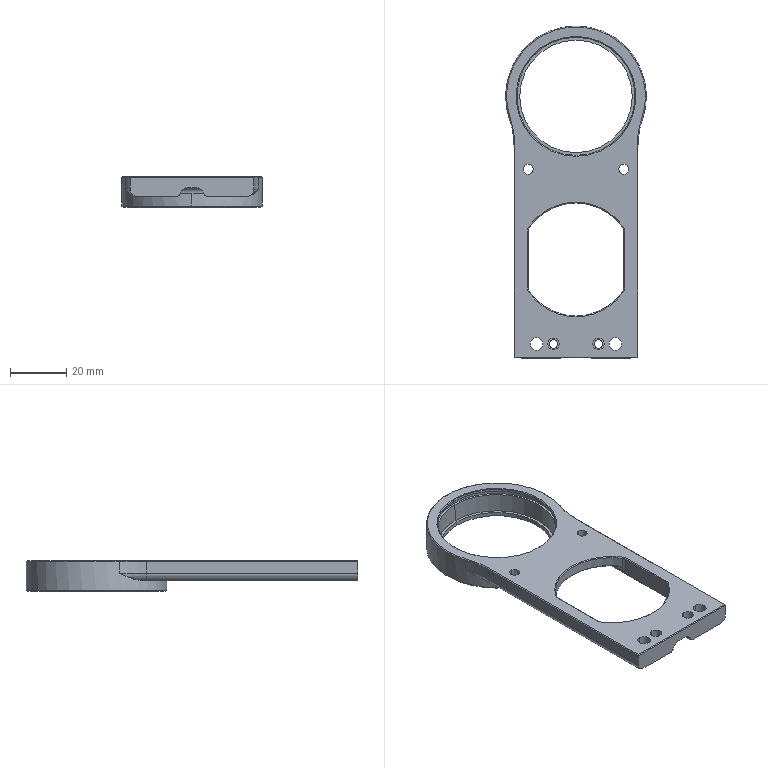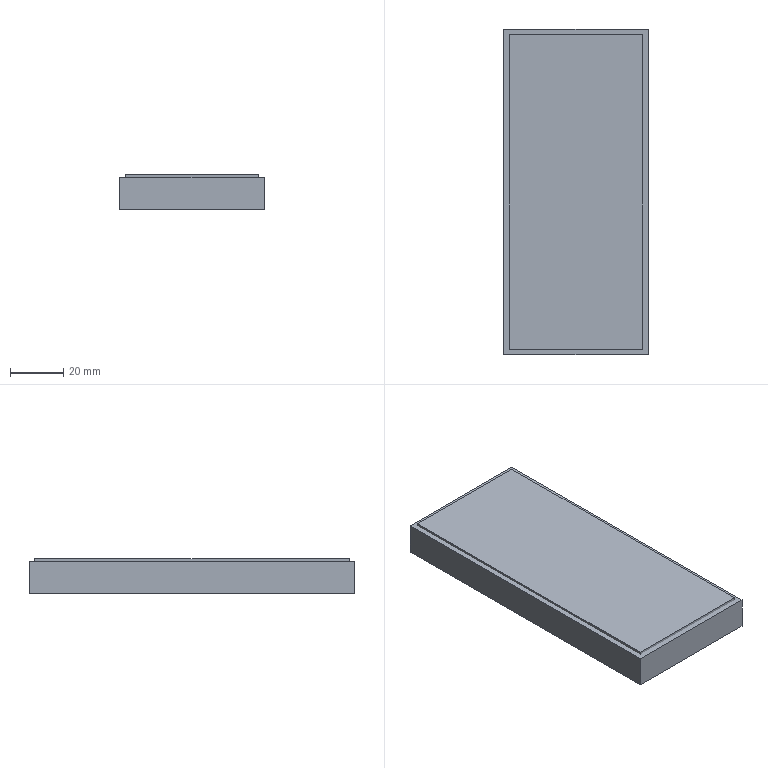CAM job | NX | 3-axis milling, drilling | part box 50 x 118 x 11 mm | stock box 54 x 122 x 13 mm
Tools:
number,name,description,diameter,corner_radius,flute_length,length,flutes
19,D80,Milling Tool-5 Parameters,80.0,0.0,50.0,75.0,2
15,D10,Milling Tool-5 Parameters,10.0,0.0,50.0,75.0,2
14,D10JING,Milling Tool-5 Parameters,10.0,0.0,50.0,75.0,2
1,D6A45,Milling Tool-5 Parameters,6.0,0.0,50.0,75.0,2
8,4.5ZT,Drilling Tool,4.5,0.0,35.0,50.0,2
16,3.0ZT,Drilling Tool,3.0,0.0,35.0,50.0,2
7,3.5ZT,Drilling Tool,3.4,0.0,35.0,50.0,2
17,D2,Milling Tool-5 Parameters,2.0,0.0,50.0,75.0,2
11,D4,Milling Tool-5 Parameters,4.0,0.0,50.0,75.0,2
18,D3R0.5,Milling Tool-5 Parameters,3.0,0.5,50.0,75.0,2
21,T6H4D1.5,Milling Tool-T Cutter,6.0,,1.5,25.0,4
Operations:
program,operation,operation_type,tool,method,geometry_group,spindle_rpm,surface_speed,feed_per_tooth,feed_cut,feed_plunge,cut_length_mm,path_length_mm,cut_time_min,machine_time_min
1,FLOOR_WALL,VolumeBased25DMillingOperation,D80,METHOD,A,5000.0,1256.0,0.12,1200.0,100.0,214.0,268.0,0.1783,0.1837
1,ZLEVEL_PROFILE,ZLevelMilling,D10,METHOD,A,9500.0,298.0,0.1842,3500.0,1000.0,4822.763,4890.763,1.409,1.416
1,PLANAR_MILL_3,PlanarMilling,D10,METHOD,A,9500.0,298.0,0.1842,3500.0,1000.0,2427.202,2623.254,1.069,1.088
1,HOLE_MILLING_COPY,CylinderMilling,D10,METHOD,A,9500.0,0.0,0.0,2500.0,1000.0,990.111,1061.111,0.3984,0.4055
1,ZLEVEL_PROFILE_COPY,ZLevelMilling,D10JING,METHOD,A,9500.0,298.0,0.0789,1500.0,1000.0,370.783,449.783,0.2567,0.2646
1,ZLEVEL_PROFILE_COPY_1_COPY,ZLevelMilling,D10JING,METHOD,A,9500.0,298.0,0.0789,1500.0,1000.0,122.302,200.302,0.0911,0.0989
1,HOLE_MILLING_COPY_COPY,CylinderMilling,D10JING,METHOD,A,9500.0,0.0,0.1053,2000.0,1000.0,1159.087,1228.112,0.5921,0.599
1,HOLE_MILLING_COPY_COPY_COPY,CylinderMilling,D10JING,METHOD,A,9500.0,0.0,0.1053,2000.0,1000.0,264.056,324.806,0.1413,0.1474
1,SPOT_DRILLING,Operation,D6A45,METHOD,A,9500.0,179.0,0.0132,250.0,0.0,28.0,288.202,0.112,0.138
1,DRILLING,Operation,4.5ZT,METHOD,A,2500.0,35.0,0.04,200.0,0.0,18.904,128.968,0.0945,0.1055
1,DRILLING_COPY,Operation,3.0ZT,METHOD,A,2500.0,35.0,0.04,200.0,0.0,24.803,128.884,0.124,0.1344
1,DRILLING_COPY_COPY,Operation,3.5ZT,METHOD,A,2500.0,35.0,0.04,200.0,0.0,25.043,147.218,0.1252,0.1374
1,ZLEVEL_PROFILE_COPY_1_COPY_1,ZLevelMilling,D4,METHOD,A,9500.0,119.0,0.1053,2000.0,1000.0,727.717,1313.287,0.5001,0.5587
1,HOLE_MILLING_1,CylinderMilling,D2,METHOD,A,9500.0,59.0,0.0553,1050.0,100.0,479.748,624.748,0.4569,0.4714
1,PLANAR_PROFILE,PlanarMilling,D6A45,METHOD,A,9500.0,179.0,0.0789,1500.0,100.0,577.995,865.461,0.3853,0.4141
1,PLANAR_PROFILE_COPY,PlanarMilling,D6A45,METHOD,A,9500.0,179.0,0.0789,1500.0,100.0,81.045,559.42,0.054,0.1019
1,PLANAR_MILL,PlanarMilling,T6H4D1.5,METHOD,A,9500.0,179.0,0.0329,1250.0,100.0,366.114,425.114,0.2929,0.2988
2,FLOOR_WALL_COPY,VolumeBased25DMillingOperation,D80,METHOD,B,5000.0,1256.0,0.12,1200.0,100.0,428.0,741.7,0.3567,0.388
2,FLOOR_WALL_COPY_COPY,VolumeBased25DMillingOperation,D80,METHOD,B,5000.0,1256.0,0.12,1200.0,100.0,214.0,268.0,0.1783,0.1837
2,FLOOR_WALL_1,VolumeBased25DMillingOperation,D10,METHOD,B,9500.0,298.0,0.1316,2500.0,1000.0,4682.065,4846.9,2.015,2.031
2,FLOOR_WALL_1_COPY,VolumeBased25DMillingOperation,D10,METHOD,B,9500.0,298.0,0.1316,2500.0,1000.0,934.411,1180.147,0.5939,0.6185
2,FLOOR_WALL_1_COPY_1_COPY_COPY,VolumeBased25DMillingOperation,D10JING,METHOD,B,9500.0,119.0,0.0632,1200.0,1000.0,1053.375,1671.004,0.8821,0.9438
2,HOLE_MILLING_2,CylinderMilling,D4,METHOD,B,9500.0,119.0,0.0658,1250.0,100.0,212.223,382.023,0.1698,0.1868
2,FLOOR_WALL_1_COPY_1,VolumeBased25DMillingOperation,D4,METHOD,B,9500.0,119.0,0.1053,2000.0,1000.0,865.886,1629.214,0.5963,0.6726
2,ZLEVEL_PROFILE_1_COPY,ZLevelMilling,D3R0.5,METHOD,B,9500.0,89.0,0.1316,2500.0,1000.0,26172.752,26608.685,10.485,10.528
2,ZLEVEL_PROFILE_1_COPY_COPY,ZLevelMilling,D3R0.5,METHOD,B,9500.0,89.0,0.1316,2500.0,1000.0,1212.83,1790.067,0.5077,0.5654
2,ZLEVEL_PROFILE_1_COPY_COPY_COPY,ZLevelMilling,D3R0.5,METHOD,B,9500.0,89.0,0.1316,2500.0,1000.0,7760.246,8077.341,3.117,3.148
2,PLANAR_MILL_2,PlanarMilling,D6A45,METHOD,B,9500.0,179.0,0.0658,1250.0,100.0,126.515,185.515,0.1012,0.1071
2,PLANAR_MILL_2_COPY,PlanarMilling,D6A45,METHOD,B,9500.0,179.0,0.0658,1250.0,100.0,166.864,225.864,0.1335,0.1394
2,PLANAR_MILL_2_COPY_1,PlanarMilling,D6A45,METHOD,B,9500.0,179.0,0.0658,1250.0,100.0,122.186,802.801,0.0977,0.1658
PROGRAM,PLANAR_MILL_1,PlanarMilling,D6A45,METHOD,NONE,9500.0,179.0,0.0658,1250.0,100.0,0.0,0.0,0.0,0.0,missing
PROGRAM,ZLEVEL_PROFILE_COPY_1,ZLevelMilling,D10,METHOD,B,9500.0,298.0,0.1842,3500.0,1000.0,1145.871,1213.671,0.3605,0.3673